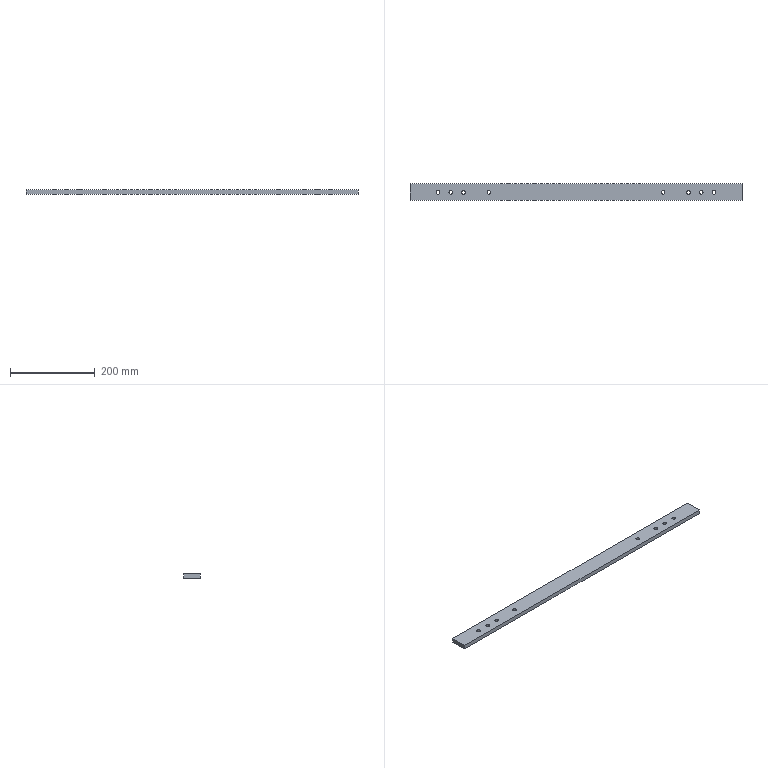Part | SolidWorks | features Extrusion 1, HoleWzd 1 | 1 solid | 22 faces | box 782 x 40 x 10 mm | volume 308260 mm3 | cylinder 16 | plane 6 | commonest cylinder face diameters 8.5 x16
STEP:
#1=CARTESIAN_POINT('',(-320.75,-0.78,0.));
#2=VERTEX_POINT('',#1);
#3=CARTESIAN_POINT('',(-329.25,-0.78,0.));
#4=VERTEX_POINT('',#3);
#5=CARTESIAN_POINT('',(-325.,-0.78,0.));
#6=DIRECTION('',(0.,0.,-1.));
#7=DIRECTION('',(-1.,0.,0.));
#8=AXIS2_PLACEMENT_3D('',#5,#6,#7);
#9=CIRCLE('',#8,4.25);
#10=EDGE_CURVE('',#2,#4,#9,.T.);
#11=ORIENTED_EDGE('',*,*,#10,.T.);
#12=CARTESIAN_POINT('',(-329.25,-0.78,10.));
#13=VERTEX_POINT('',#12);
#14=CARTESIAN_POINT('',(-329.25,-0.78,10.));
#15=DIRECTION('',(0.,0.,1.));
#16=VECTOR('',#15,1000.);
#17=LINE('',#14,#16);
#18=EDGE_CURVE('',#4,#13,#17,.T.);
#19=ORIENTED_EDGE('',*,*,#18,.T.);
#20=CARTESIAN_POINT('',(-320.75,-0.78,10.));
#21=VERTEX_POINT('',#20);
#22=CARTESIAN_POINT('',(-325.,-0.78,10.));
#23=DIRECTION('',(0.,0.,1.));
#24=DIRECTION('',(1.,0.,0.));
#25=AXIS2_PLACEMENT_3D('',#22,#23,#24);
#26=CIRCLE('',#25,4.25);
#27=EDGE_CURVE('',#13,#21,#26,.T.);
#28=ORIENTED_EDGE('',*,*,#27,.T.);
#29=CARTESIAN_POINT('',(-320.75,-0.78,10.));
#30=DIRECTION('',(0.,0.,1.));
#31=VECTOR('',#30,1000.);
#32=LINE('',#29,#31);
#33=EDGE_CURVE('',#2,#21,#32,.T.);
#34=ORIENTED_EDGE('',*,*,#33,.F.);
#35=EDGE_LOOP('',(#11,#19,#28,#34));
#36=FACE_OUTER_BOUND('',#35,.T.);
#37=CARTESIAN_POINT('',(-325.,-0.78,10.));
#38=DIRECTION('',(0.,0.,1.));
#39=DIRECTION('',(1.,0.,0.));
#40=AXIS2_PLACEMENT_3D('',#37,#38,#39);
#41=CYLINDRICAL_SURFACE('',#40,4.25);
#42=ADVANCED_FACE('',(#36),#41,.F.);
#43=CARTESIAN_POINT('',(-290.75,-0.78,0.));
#44=VERTEX_POINT('',#43);
#45=CARTESIAN_POINT('',(-299.25,-0.78,0.));
#46=VERTEX_POINT('',#45);
#47=CARTESIAN_POINT('',(-295.,-0.78,0.));
#48=DIRECTION('',(0.,0.,-1.));
#49=DIRECTION('',(-1.,0.,0.));
#50=AXIS2_PLACEMENT_3D('',#47,#48,#49);
#51=CIRCLE('',#50,4.25);
#52=EDGE_CURVE('',#44,#46,#51,.T.);
#53=ORIENTED_EDGE('',*,*,#52,.T.);
#54=CARTESIAN_POINT('',(-299.25,-0.78,10.));
#55=VERTEX_POINT('',#54);
#56=CARTESIAN_POINT('',(-299.25,-0.78,10.));
#57=DIRECTION('',(0.,0.,1.));
#58=VECTOR('',#57,1000.);
#59=LINE('',#56,#58);
#60=EDGE_CURVE('',#46,#55,#59,.T.);
#61=ORIENTED_EDGE('',*,*,#60,.T.);
#62=CARTESIAN_POINT('',(-290.75,-0.78,10.));
#63=VERTEX_POINT('',#62);
#64=CARTESIAN_POINT('',(-295.,-0.78,10.));
#65=DIRECTION('',(0.,0.,1.));
#66=DIRECTION('',(1.,0.,0.));
#67=AXIS2_PLACEMENT_3D('',#64,#65,#66);
#68=CIRCLE('',#67,4.25);
#69=EDGE_CURVE('',#55,#63,#68,.T.);
#70=ORIENTED_EDGE('',*,*,#69,.T.);
#71=CARTESIAN_POINT('',(-290.75,-0.78,10.));
#72=DIRECTION('',(0.,0.,1.));
#73=VECTOR('',#72,1000.);
#74=LINE('',#71,#73);
#75=EDGE_CURVE('',#44,#63,#74,.T.);
#76=ORIENTED_EDGE('',*,*,#75,.F.);
#77=EDGE_LOOP('',(#53,#61,#70,#76));
#78=FACE_OUTER_BOUND('',#77,.T.);
#79=CARTESIAN_POINT('',(-295.,-0.78,10.));
#80=DIRECTION('',(0.,0.,1.));
#81=DIRECTION('',(1.,0.,0.));
#82=AXIS2_PLACEMENT_3D('',#79,#80,#81);
#83=CYLINDRICAL_SURFACE('',#82,4.25);
#84=ADVANCED_FACE('',(#78),#83,.F.);
#85=CARTESIAN_POINT('',(-260.75,-0.78,0.));
#86=VERTEX_POINT('',#85);
#87=CARTESIAN_POINT('',(-269.25,-0.78,0.));
#88=VERTEX_POINT('',#87);
#89=CARTESIAN_POINT('',(-265.,-0.78,0.));
#90=DIRECTION('',(0.,0.,-1.));
#91=DIRECTION('',(-1.,0.,0.));
#92=AXIS2_PLACEMENT_3D('',#89,#90,#91);
#93=CIRCLE('',#92,4.25);
#94=EDGE_CURVE('',#86,#88,#93,.T.);
#95=ORIENTED_EDGE('',*,*,#94,.T.);
#96=CARTESIAN_POINT('',(-269.25,-0.78,10.));
#97=VERTEX_POINT('',#96);
#98=CARTESIAN_POINT('',(-269.25,-0.78,10.));
#99=DIRECTION('',(0.,0.,1.));
#100=VECTOR('',#99,1000.);
#101=LINE('',#98,#100);
#102=EDGE_CURVE('',#88,#97,#101,.T.);
#103=ORIENTED_EDGE('',*,*,#102,.T.);
#104=CARTESIAN_POINT('',(-260.75,-0.78,10.));
#105=VERTEX_POINT('',#104);
#106=CARTESIAN_POINT('',(-265.,-0.78,10.));
#107=DIRECTION('',(0.,0.,1.));
#108=DIRECTION('',(1.,0.,0.));
#109=AXIS2_PLACEMENT_3D('',#106,#107,#108);
#110=CIRCLE('',#109,4.25);
#111=EDGE_CURVE('',#97,#105,#110,.T.);
#112=ORIENTED_EDGE('',*,*,#111,.T.);
#113=CARTESIAN_POINT('',(-260.75,-0.78,10.));
#114=DIRECTION('',(0.,0.,1.));
#115=VECTOR('',#114,1000.);
#116=LINE('',#113,#115);
#117=EDGE_CURVE('',#86,#105,#116,.T.);
#118=ORIENTED_EDGE('',*,*,#117,.F.);
#119=EDGE_LOOP('',(#95,#103,#112,#118));
#120=FACE_OUTER_BOUND('',#119,.T.);
#121=CARTESIAN_POINT('',(-265.,-0.78,10.));
#122=DIRECTION('',(0.,0.,1.));
#123=DIRECTION('',(1.,0.,0.));
#124=AXIS2_PLACEMENT_3D('',#121,#122,#123);
#125=CYLINDRICAL_SURFACE('',#124,4.25);
#126=ADVANCED_FACE('',(#120),#125,.F.);
#127=CARTESIAN_POINT('',(-200.75,-0.78,0.));
#128=VERTEX_POINT('',#127);
#129=CARTESIAN_POINT('',(-209.25,-0.78,0.));
#130=VERTEX_POINT('',#129);
#131=CARTESIAN_POINT('',(-205.,-0.78,0.));
#132=DIRECTION('',(0.,0.,-1.));
#133=DIRECTION('',(-1.,0.,0.));
#134=AXIS2_PLACEMENT_3D('',#131,#132,#133);
#135=CIRCLE('',#134,4.25);
#136=EDGE_CURVE('',#128,#130,#135,.T.);
#137=ORIENTED_EDGE('',*,*,#136,.T.);
#138=CARTESIAN_POINT('',(-209.25,-0.78,10.));
#139=VERTEX_POINT('',#138);
#140=CARTESIAN_POINT('',(-209.25,-0.78,10.));
#141=DIRECTION('',(0.,0.,1.));
#142=VECTOR('',#141,1000.);
#143=LINE('',#140,#142);
#144=EDGE_CURVE('',#130,#139,#143,.T.);
#145=ORIENTED_EDGE('',*,*,#144,.T.);
#146=CARTESIAN_POINT('',(-200.75,-0.78,10.));
#147=VERTEX_POINT('',#146);
#148=CARTESIAN_POINT('',(-205.,-0.78,10.));
#149=DIRECTION('',(0.,0.,1.));
#150=DIRECTION('',(1.,0.,0.));
#151=AXIS2_PLACEMENT_3D('',#148,#149,#150);
#152=CIRCLE('',#151,4.25);
#153=EDGE_CURVE('',#139,#147,#152,.T.);
#154=ORIENTED_EDGE('',*,*,#153,.T.);
#155=CARTESIAN_POINT('',(-200.75,-0.78,10.));
#156=DIRECTION('',(0.,0.,1.));
#157=VECTOR('',#156,1000.);
#158=LINE('',#155,#157);
#159=EDGE_CURVE('',#128,#147,#158,.T.);
#160=ORIENTED_EDGE('',*,*,#159,.F.);
#161=EDGE_LOOP('',(#137,#145,#154,#160));
#162=FACE_OUTER_BOUND('',#161,.T.);
#163=CARTESIAN_POINT('',(-205.,-0.78,10.));
#164=DIRECTION('',(0.,0.,1.));
#165=DIRECTION('',(1.,0.,0.));
#166=AXIS2_PLACEMENT_3D('',#163,#164,#165);
#167=CYLINDRICAL_SURFACE('',#166,4.25);
#168=ADVANCED_FACE('',(#162),#167,.F.);
#169=CARTESIAN_POINT('',(209.25,-0.78,0.));
#170=VERTEX_POINT('',#169);
#171=CARTESIAN_POINT('',(200.75,-0.78,0.));
#172=VERTEX_POINT('',#171);
#173=CARTESIAN_POINT('',(205.,-0.78,0.));
#174=DIRECTION('',(0.,0.,-1.));
#175=DIRECTION('',(-1.,0.,0.));
#176=AXIS2_PLACEMENT_3D('',#173,#174,#175);
#177=CIRCLE('',#176,4.25);
#178=EDGE_CURVE('',#170,#172,#177,.T.);
#179=ORIENTED_EDGE('',*,*,#178,.T.);
#180=CARTESIAN_POINT('',(200.75,-0.78,10.));
#181=VERTEX_POINT('',#180);
#182=CARTESIAN_POINT('',(200.75,-0.78,10.));
#183=DIRECTION('',(0.,0.,1.));
#184=VECTOR('',#183,1000.);
#185=LINE('',#182,#184);
#186=EDGE_CURVE('',#172,#181,#185,.T.);
#187=ORIENTED_EDGE('',*,*,#186,.T.);
#188=CARTESIAN_POINT('',(209.25,-0.78,10.));
#189=VERTEX_POINT('',#188);
#190=CARTESIAN_POINT('',(205.,-0.78,10.));
#191=DIRECTION('',(0.,0.,1.));
#192=DIRECTION('',(1.,0.,0.));
#193=AXIS2_PLACEMENT_3D('',#190,#191,#192);
#194=CIRCLE('',#193,4.25);
#195=EDGE_CURVE('',#181,#189,#194,.T.);
#196=ORIENTED_EDGE('',*,*,#195,.T.);
#197=CARTESIAN_POINT('',(209.25,-0.78,10.));
#198=DIRECTION('',(0.,0.,1.));
#199=VECTOR('',#198,1000.);
#200=LINE('',#197,#199);
#201=EDGE_CURVE('',#170,#189,#200,.T.);
#202=ORIENTED_EDGE('',*,*,#201,.F.);
#203=EDGE_LOOP('',(#179,#187,#196,#202));
#204=FACE_OUTER_BOUND('',#203,.T.);
#205=CARTESIAN_POINT('',(205.,-0.78,10.));
#206=DIRECTION('',(0.,0.,1.));
#207=DIRECTION('',(1.,0.,0.));
#208=AXIS2_PLACEMENT_3D('',#205,#206,#207);
#209=CYLINDRICAL_SURFACE('',#208,4.25);
#210=ADVANCED_FACE('',(#204),#209,.F.);
#211=CARTESIAN_POINT('',(269.25,-0.78,0.));
#212=VERTEX_POINT('',#211);
#213=CARTESIAN_POINT('',(260.75,-0.78,0.));
#214=VERTEX_POINT('',#213);
#215=CARTESIAN_POINT('',(265.,-0.78,0.));
#216=DIRECTION('',(0.,0.,-1.));
#217=DIRECTION('',(-1.,0.,0.));
#218=AXIS2_PLACEMENT_3D('',#215,#216,#217);
#219=CIRCLE('',#218,4.25);
#220=EDGE_CURVE('',#212,#214,#219,.T.);
#221=ORIENTED_EDGE('',*,*,#220,.T.);
#222=CARTESIAN_POINT('',(260.75,-0.78,10.));
#223=VERTEX_POINT('',#222);
#224=CARTESIAN_POINT('',(260.75,-0.78,10.));
#225=DIRECTION('',(0.,0.,1.));
#226=VECTOR('',#225,1000.);
#227=LINE('',#224,#226);
#228=EDGE_CURVE('',#214,#223,#227,.T.);
#229=ORIENTED_EDGE('',*,*,#228,.T.);
#230=CARTESIAN_POINT('',(269.25,-0.78,10.));
#231=VERTEX_POINT('',#230);
#232=CARTESIAN_POINT('',(265.,-0.78,10.));
#233=DIRECTION('',(0.,0.,1.));
#234=DIRECTION('',(1.,0.,0.));
#235=AXIS2_PLACEMENT_3D('',#232,#233,#234);
#236=CIRCLE('',#235,4.25);
#237=EDGE_CURVE('',#223,#231,#236,.T.);
#238=ORIENTED_EDGE('',*,*,#237,.T.);
#239=CARTESIAN_POINT('',(269.25,-0.78,10.));
#240=DIRECTION('',(0.,0.,1.));
#241=VECTOR('',#240,1000.);
#242=LINE('',#239,#241);
#243=EDGE_CURVE('',#212,#231,#242,.T.);
#244=ORIENTED_EDGE('',*,*,#243,.F.);
#245=EDGE_LOOP('',(#221,#229,#238,#244));
#246=FACE_OUTER_BOUND('',#245,.T.);
#247=CARTESIAN_POINT('',(265.,-0.78,10.));
#248=DIRECTION('',(0.,0.,1.));
#249=DIRECTION('',(1.,0.,0.));
#250=AXIS2_PLACEMENT_3D('',#247,#248,#249);
#251=CYLINDRICAL_SURFACE('',#250,4.25);
#252=ADVANCED_FACE('',(#246),#251,.F.);
#253=CARTESIAN_POINT('',(299.25,-0.78,0.));
#254=VERTEX_POINT('',#253);
#255=CARTESIAN_POINT('',(290.75,-0.78,0.));
#256=VERTEX_POINT('',#255);
#257=CARTESIAN_POINT('',(295.,-0.78,0.));
#258=DIRECTION('',(0.,0.,-1.));
#259=DIRECTION('',(-1.,0.,0.));
#260=AXIS2_PLACEMENT_3D('',#257,#258,#259);
#261=CIRCLE('',#260,4.25);
#262=EDGE_CURVE('',#254,#256,#261,.T.);
#263=ORIENTED_EDGE('',*,*,#262,.T.);
#264=CARTESIAN_POINT('',(290.75,-0.78,10.));
#265=VERTEX_POINT('',#264);
#266=CARTESIAN_POINT('',(290.75,-0.78,10.));
#267=DIRECTION('',(0.,0.,1.));
#268=VECTOR('',#267,1000.);
#269=LINE('',#266,#268);
#270=EDGE_CURVE('',#256,#265,#269,.T.);
#271=ORIENTED_EDGE('',*,*,#270,.T.);
#272=CARTESIAN_POINT('',(299.25,-0.78,10.));
#273=VERTEX_POINT('',#272);
#274=CARTESIAN_POINT('',(295.,-0.78,10.));
#275=DIRECTION('',(0.,0.,1.));
#276=DIRECTION('',(1.,0.,0.));
#277=AXIS2_PLACEMENT_3D('',#274,#275,#276);
#278=CIRCLE('',#277,4.25);
#279=EDGE_CURVE('',#265,#273,#278,.T.);
#280=ORIENTED_EDGE('',*,*,#279,.T.);
#281=CARTESIAN_POINT('',(299.25,-0.78,10.));
#282=DIRECTION('',(0.,0.,1.));
#283=VECTOR('',#282,1000.);
#284=LINE('',#281,#283);
#285=EDGE_CURVE('',#254,#273,#284,.T.);
#286=ORIENTED_EDGE('',*,*,#285,.F.);
#287=EDGE_LOOP('',(#263,#271,#280,#286));
#288=FACE_OUTER_BOUND('',#287,.T.);
#289=CARTESIAN_POINT('',(295.,-0.78,10.));
#290=DIRECTION('',(0.,0.,1.));
#291=DIRECTION('',(1.,0.,0.));
#292=AXIS2_PLACEMENT_3D('',#289,#290,#291);
#293=CYLINDRICAL_SURFACE('',#292,4.25);
#294=ADVANCED_FACE('',(#288),#293,.F.);
#295=CARTESIAN_POINT('',(329.25,-0.78,0.));
#296=VERTEX_POINT('',#295);
#297=CARTESIAN_POINT('',(320.75,-0.78,0.));
#298=VERTEX_POINT('',#297);
#299=CARTESIAN_POINT('',(325.,-0.78,0.));
#300=DIRECTION('',(0.,0.,-1.));
#301=DIRECTION('',(-1.,0.,0.));
#302=AXIS2_PLACEMENT_3D('',#299,#300,#301);
#303=CIRCLE('',#302,4.25);
#304=EDGE_CURVE('',#296,#298,#303,.T.);
#305=ORIENTED_EDGE('',*,*,#304,.T.);
#306=CARTESIAN_POINT('',(320.75,-0.78,10.));
#307=VERTEX_POINT('',#306);
#308=CARTESIAN_POINT('',(320.75,-0.78,10.));
#309=DIRECTION('',(0.,0.,1.));
#310=VECTOR('',#309,1000.);
#311=LINE('',#308,#310);
#312=EDGE_CURVE('',#298,#307,#311,.T.);
#313=ORIENTED_EDGE('',*,*,#312,.T.);
#314=CARTESIAN_POINT('',(329.25,-0.78,10.));
#315=VERTEX_POINT('',#314);
#316=CARTESIAN_POINT('',(325.,-0.78,10.));
#317=DIRECTION('',(0.,0.,1.));
#318=DIRECTION('',(1.,0.,0.));
#319=AXIS2_PLACEMENT_3D('',#316,#317,#318);
#320=CIRCLE('',#319,4.25);
#321=EDGE_CURVE('',#307,#315,#320,.T.);
#322=ORIENTED_EDGE('',*,*,#321,.T.);
#323=CARTESIAN_POINT('',(329.25,-0.78,10.));
#324=DIRECTION('',(0.,0.,1.));
#325=VECTOR('',#324,1000.);
#326=LINE('',#323,#325);
#327=EDGE_CURVE('',#296,#315,#326,.T.);
#328=ORIENTED_EDGE('',*,*,#327,.F.);
#329=EDGE_LOOP('',(#305,#313,#322,#328));
#330=FACE_OUTER_BOUND('',#329,.T.);
#331=CARTESIAN_POINT('',(325.,-0.78,10.));
#332=DIRECTION('',(0.,0.,1.));
#333=DIRECTION('',(1.,0.,0.));
#334=AXIS2_PLACEMENT_3D('',#331,#332,#333);
#335=CYLINDRICAL_SURFACE('',#334,4.25);
#336=ADVANCED_FACE('',(#330),#335,.F.);
#337=CARTESIAN_POINT('',(-391.,20.,0.));
#338=VERTEX_POINT('',#337);
#339=CARTESIAN_POINT('',(-391.,-20.,0.));
#340=VERTEX_POINT('',#339);
#341=CARTESIAN_POINT('',(-391.,20.,0.));
#342=DIRECTION('',(0.,-1.,0.));
#343=VECTOR('',#342,1000.);
#344=LINE('',#341,#343);
#345=EDGE_CURVE('',#338,#340,#344,.T.);
#346=ORIENTED_EDGE('',*,*,#345,.T.);
#347=CARTESIAN_POINT('',(-391.,-20.,10.));
#348=VERTEX_POINT('',#347);
#349=CARTESIAN_POINT('',(-391.,-20.,10.));
#350=DIRECTION('',(0.,0.,-1.));
#351=VECTOR('',#350,1000.);
#352=LINE('',#349,#351);
#353=EDGE_CURVE('',#348,#340,#352,.T.);
#354=ORIENTED_EDGE('',*,*,#353,.F.);
#355=CARTESIAN_POINT('',(-391.,20.,10.));
#356=VERTEX_POINT('',#355);
#357=CARTESIAN_POINT('',(-391.,20.,10.));
#358=DIRECTION('',(0.,-1.,0.));
#359=VECTOR('',#358,1000.);
#360=LINE('',#357,#359);
#361=EDGE_CURVE('',#356,#348,#360,.T.);
#362=ORIENTED_EDGE('',*,*,#361,.F.);
#363=CARTESIAN_POINT('',(-391.,20.,10.));
#364=DIRECTION('',(0.,0.,-1.));
#365=VECTOR('',#364,1000.);
#366=LINE('',#363,#365);
#367=EDGE_CURVE('',#356,#338,#366,.T.);
#368=ORIENTED_EDGE('',*,*,#367,.T.);
#369=EDGE_LOOP('',(#346,#354,#362,#368));
#370=FACE_OUTER_BOUND('',#369,.T.);
#371=CARTESIAN_POINT('',(-391.,20.,10.));
#372=DIRECTION('',(1.,0.,0.));
#373=DIRECTION('',(0.,0.,-1.));
#374=AXIS2_PLACEMENT_3D('',#371,#372,#373);
#375=PLANE('',#374);
#376=ADVANCED_FACE('',(#370),#375,.F.);
#377=CARTESIAN_POINT('',(391.,-20.,0.));
#378=VERTEX_POINT('',#377);
#379=CARTESIAN_POINT('',(391.,-20.,0.));
#380=DIRECTION('',(1.,0.,0.));
#381=VECTOR('',#380,1000.);
#382=LINE('',#379,#381);
#383=EDGE_CURVE('',#340,#378,#382,.T.);
#384=ORIENTED_EDGE('',*,*,#383,.T.);
#385=CARTESIAN_POINT('',(391.,-20.,10.));
#386=VERTEX_POINT('',#385);
#387=CARTESIAN_POINT('',(391.,-20.,10.));
#388=DIRECTION('',(0.,0.,-1.));
#389=VECTOR('',#388,1000.);
#390=LINE('',#387,#389);
#391=EDGE_CURVE('',#386,#378,#390,.T.);
#392=ORIENTED_EDGE('',*,*,#391,.F.);
#393=CARTESIAN_POINT('',(391.,-20.,10.));
#394=DIRECTION('',(1.,0.,0.));
#395=VECTOR('',#394,1000.);
#396=LINE('',#393,#395);
#397=EDGE_CURVE('',#348,#386,#396,.T.);
#398=ORIENTED_EDGE('',*,*,#397,.F.);
#399=ORIENTED_EDGE('',*,*,#353,.T.);
#400=EDGE_LOOP('',(#384,#392,#398,#399));
#401=FACE_OUTER_BOUND('',#400,.T.);
#402=CARTESIAN_POINT('',(391.,-20.,10.));
#403=DIRECTION('',(0.,1.,0.));
#404=DIRECTION('',(-1.,0.,0.));
#405=AXIS2_PLACEMENT_3D('',#402,#403,#404);
#406=PLANE('',#405);
#407=ADVANCED_FACE('',(#401),#406,.F.);
#408=CARTESIAN_POINT('',(391.,20.,0.));
#409=VERTEX_POINT('',#408);
#410=CARTESIAN_POINT('',(391.,20.,0.));
#411=DIRECTION('',(0.,1.,0.));
#412=VECTOR('',#411,1000.);
#413=LINE('',#410,#412);
#414=EDGE_CURVE('',#378,#409,#413,.T.);
#415=ORIENTED_EDGE('',*,*,#414,.T.);
#416=CARTESIAN_POINT('',(391.,20.,10.));
#417=VERTEX_POINT('',#416);
#418=CARTESIAN_POINT('',(391.,20.,10.));
#419=DIRECTION('',(0.,0.,-1.));
#420=VECTOR('',#419,1000.);
#421=LINE('',#418,#420);
#422=EDGE_CURVE('',#417,#409,#421,.T.);
#423=ORIENTED_EDGE('',*,*,#422,.F.);
#424=CARTESIAN_POINT('',(391.,20.,10.));
#425=DIRECTION('',(0.,1.,0.));
#426=VECTOR('',#425,1000.);
#427=LINE('',#424,#426);
#428=EDGE_CURVE('',#386,#417,#427,.T.);
#429=ORIENTED_EDGE('',*,*,#428,.F.);
#430=ORIENTED_EDGE('',*,*,#391,.T.);
#431=EDGE_LOOP('',(#415,#423,#429,#430));
#432=FACE_OUTER_BOUND('',#431,.T.);
#433=CARTESIAN_POINT('',(391.,20.,10.));
#434=DIRECTION('',(-1.,0.,0.));
#435=DIRECTION('',(0.,0.,1.));
#436=AXIS2_PLACEMENT_3D('',#433,#434,#435);
#437=PLANE('',#436);
#438=ADVANCED_FACE('',(#432),#437,.F.);
#439=CARTESIAN_POINT('',(391.,20.,0.));
#440=DIRECTION('',(-1.,0.,0.));
#441=VECTOR('',#440,1000.);
#442=LINE('',#439,#441);
#443=EDGE_CURVE('',#409,#338,#442,.T.);
#444=ORIENTED_EDGE('',*,*,#443,.T.);
#445=ORIENTED_EDGE('',*,*,#367,.F.);
#446=CARTESIAN_POINT('',(391.,20.,10.));
#447=DIRECTION('',(-1.,0.,0.));
#448=VECTOR('',#447,1000.);
#449=LINE('',#446,#448);
#450=EDGE_CURVE('',#417,#356,#449,.T.);
#451=ORIENTED_EDGE('',*,*,#450,.F.);
#452=ORIENTED_EDGE('',*,*,#422,.T.);
#453=EDGE_LOOP('',(#444,#445,#451,#452));
#454=FACE_OUTER_BOUND('',#453,.T.);
#455=CARTESIAN_POINT('',(391.,20.,10.));
#456=DIRECTION('',(0.,-1.,0.));
#457=DIRECTION('',(1.,0.,0.));
#458=AXIS2_PLACEMENT_3D('',#455,#456,#457);
#459=PLANE('',#458);
#460=ADVANCED_FACE('',(#454),#459,.F.);
#461=CARTESIAN_POINT('',(-325.,-0.78,10.));
#462=DIRECTION('',(0.,0.,1.));
#463=DIRECTION('',(1.,0.,0.));
#464=AXIS2_PLACEMENT_3D('',#461,#462,#463);
#465=CIRCLE('',#464,4.25);
#466=EDGE_CURVE('',#21,#13,#465,.T.);
#467=ORIENTED_EDGE('',*,*,#466,.F.);
#468=ORIENTED_EDGE('',*,*,#27,.F.);
#469=EDGE_LOOP('',(#467,#468));
#470=FACE_BOUND('',#469,.T.);
#471=CARTESIAN_POINT('',(-295.,-0.78,10.));
#472=DIRECTION('',(0.,0.,1.));
#473=DIRECTION('',(1.,0.,0.));
#474=AXIS2_PLACEMENT_3D('',#471,#472,#473);
#475=CIRCLE('',#474,4.25);
#476=EDGE_CURVE('',#63,#55,#475,.T.);
#477=ORIENTED_EDGE('',*,*,#476,.F.);
#478=ORIENTED_EDGE('',*,*,#69,.F.);
#479=EDGE_LOOP('',(#477,#478));
#480=FACE_BOUND('',#479,.T.);
#481=CARTESIAN_POINT('',(-265.,-0.78,10.));
#482=DIRECTION('',(0.,0.,1.));
#483=DIRECTION('',(1.,0.,0.));
#484=AXIS2_PLACEMENT_3D('',#481,#482,#483);
#485=CIRCLE('',#484,4.25);
#486=EDGE_CURVE('',#105,#97,#485,.T.);
#487=ORIENTED_EDGE('',*,*,#486,.F.);
#488=ORIENTED_EDGE('',*,*,#111,.F.);
#489=EDGE_LOOP('',(#487,#488));
#490=FACE_BOUND('',#489,.T.);
#491=CARTESIAN_POINT('',(-205.,-0.78,10.));
#492=DIRECTION('',(0.,0.,1.));
#493=DIRECTION('',(1.,0.,0.));
#494=AXIS2_PLACEMENT_3D('',#491,#492,#493);
#495=CIRCLE('',#494,4.25);
#496=EDGE_CURVE('',#147,#139,#495,.T.);
#497=ORIENTED_EDGE('',*,*,#496,.F.);
#498=ORIENTED_EDGE('',*,*,#153,.F.);
#499=EDGE_LOOP('',(#497,#498));
#500=FACE_BOUND('',#499,.T.);
#501=CARTESIAN_POINT('',(205.,-0.78,10.));
#502=DIRECTION('',(0.,0.,1.));
#503=DIRECTION('',(1.,0.,0.));
#504=AXIS2_PLACEMENT_3D('',#501,#502,#503);
#505=CIRCLE('',#504,4.25);
#506=EDGE_CURVE('',#189,#181,#505,.T.);
#507=ORIENTED_EDGE('',*,*,#506,.F.);
#508=ORIENTED_EDGE('',*,*,#195,.F.);
#509=EDGE_LOOP('',(#507,#508));
#510=FACE_BOUND('',#509,.T.);
#511=CARTESIAN_POINT('',(265.,-0.78,10.));
#512=DIRECTION('',(0.,0.,1.));
#513=DIRECTION('',(1.,0.,0.));
#514=AXIS2_PLACEMENT_3D('',#511,#512,#513);
#515=CIRCLE('',#514,4.25);
#516=EDGE_CURVE('',#231,#223,#515,.T.);
#517=ORIENTED_EDGE('',*,*,#516,.F.);
#518=ORIENTED_EDGE('',*,*,#237,.F.);
#519=EDGE_LOOP('',(#517,#518));
#520=FACE_BOUND('',#519,.T.);
#521=CARTESIAN_POINT('',(295.,-0.78,10.));
#522=DIRECTION('',(0.,0.,1.));
#523=DIRECTION('',(1.,0.,0.));
#524=AXIS2_PLACEMENT_3D('',#521,#522,#523);
#525=CIRCLE('',#524,4.25);
#526=EDGE_CURVE('',#273,#265,#525,.T.);
#527=ORIENTED_EDGE('',*,*,#526,.F.);
#528=ORIENTED_EDGE('',*,*,#279,.F.);
#529=EDGE_LOOP('',(#527,#528));
#530=FACE_BOUND('',#529,.T.);
#531=CARTESIAN_POINT('',(325.,-0.78,10.));
#532=DIRECTION('',(0.,0.,1.));
#533=DIRECTION('',(1.,0.,0.));
#534=AXIS2_PLACEMENT_3D('',#531,#532,#533);
#535=CIRCLE('',#534,4.25);
#536=EDGE_CURVE('',#315,#307,#535,.T.);
#537=ORIENTED_EDGE('',*,*,#536,.F.);
#538=ORIENTED_EDGE('',*,*,#321,.F.);
#539=EDGE_LOOP('',(#537,#538));
#540=FACE_BOUND('',#539,.T.);
#541=ORIENTED_EDGE('',*,*,#361,.T.);
#542=ORIENTED_EDGE('',*,*,#397,.T.);
#543=ORIENTED_EDGE('',*,*,#428,.T.);
#544=ORIENTED_EDGE('',*,*,#450,.T.);
#545=EDGE_LOOP('',(#541,#542,#543,#544));
#546=FACE_OUTER_BOUND('',#545,.T.);
#547=CARTESIAN_POINT('',(0.,0.,10.));
#548=DIRECTION('',(0.,0.,-1.));
#549=DIRECTION('',(-1.,0.,0.));
#550=AXIS2_PLACEMENT_3D('',#547,#548,#549);
#551=PLANE('',#550);
#552=ADVANCED_FACE('',(#470,#480,#490,#500,#510,#520,#530,#540,#546),#551,.F.);
#553=ORIENTED_EDGE('',*,*,#10,.F.);
#554=CARTESIAN_POINT('',(-325.,-0.78,0.));
#555=DIRECTION('',(0.,0.,-1.));
#556=DIRECTION('',(-1.,0.,0.));
#557=AXIS2_PLACEMENT_3D('',#554,#555,#556);
#558=CIRCLE('',#557,4.25);
#559=EDGE_CURVE('',#4,#2,#558,.T.);
#560=ORIENTED_EDGE('',*,*,#559,.F.);
#561=EDGE_LOOP('',(#553,#560));
#562=FACE_BOUND('',#561,.T.);
#563=ORIENTED_EDGE('',*,*,#52,.F.);
#564=CARTESIAN_POINT('',(-295.,-0.78,0.));
#565=DIRECTION('',(0.,0.,-1.));
#566=DIRECTION('',(-1.,0.,0.));
#567=AXIS2_PLACEMENT_3D('',#564,#565,#566);
#568=CIRCLE('',#567,4.25);
#569=EDGE_CURVE('',#46,#44,#568,.T.);
#570=ORIENTED_EDGE('',*,*,#569,.F.);
#571=EDGE_LOOP('',(#563,#570));
#572=FACE_BOUND('',#571,.T.);
#573=ORIENTED_EDGE('',*,*,#94,.F.);
#574=CARTESIAN_POINT('',(-265.,-0.78,0.));
#575=DIRECTION('',(0.,0.,-1.));
#576=DIRECTION('',(-1.,0.,0.));
#577=AXIS2_PLACEMENT_3D('',#574,#575,#576);
#578=CIRCLE('',#577,4.25);
#579=EDGE_CURVE('',#88,#86,#578,.T.);
#580=ORIENTED_EDGE('',*,*,#579,.F.);
#581=EDGE_LOOP('',(#573,#580));
#582=FACE_BOUND('',#581,.T.);
#583=ORIENTED_EDGE('',*,*,#136,.F.);
#584=CARTESIAN_POINT('',(-205.,-0.78,0.));
#585=DIRECTION('',(0.,0.,-1.));
#586=DIRECTION('',(-1.,0.,0.));
#587=AXIS2_PLACEMENT_3D('',#584,#585,#586);
#588=CIRCLE('',#587,4.25);
#589=EDGE_CURVE('',#130,#128,#588,.T.);
#590=ORIENTED_EDGE('',*,*,#589,.F.);
#591=EDGE_LOOP('',(#583,#590));
#592=FACE_BOUND('',#591,.T.);
#593=ORIENTED_EDGE('',*,*,#178,.F.);
#594=CARTESIAN_POINT('',(205.,-0.78,0.));
#595=DIRECTION('',(0.,0.,-1.));
#596=DIRECTION('',(-1.,0.,0.));
#597=AXIS2_PLACEMENT_3D('',#594,#595,#596);
#598=CIRCLE('',#597,4.25);
#599=EDGE_CURVE('',#172,#170,#598,.T.);
#600=ORIENTED_EDGE('',*,*,#599,.F.);
#601=EDGE_LOOP('',(#593,#600));
#602=FACE_BOUND('',#601,.T.);
#603=ORIENTED_EDGE('',*,*,#220,.F.);
#604=CARTESIAN_POINT('',(265.,-0.78,0.));
#605=DIRECTION('',(0.,0.,-1.));
#606=DIRECTION('',(-1.,0.,0.));
#607=AXIS2_PLACEMENT_3D('',#604,#605,#606);
#608=CIRCLE('',#607,4.25);
#609=EDGE_CURVE('',#214,#212,#608,.T.);
#610=ORIENTED_EDGE('',*,*,#609,.F.);
#611=EDGE_LOOP('',(#603,#610));
#612=FACE_BOUND('',#611,.T.);
#613=ORIENTED_EDGE('',*,*,#262,.F.);
#614=CARTESIAN_POINT('',(295.,-0.78,0.));
#615=DIRECTION('',(0.,0.,-1.));
#616=DIRECTION('',(-1.,0.,0.));
#617=AXIS2_PLACEMENT_3D('',#614,#615,#616);
#618=CIRCLE('',#617,4.25);
#619=EDGE_CURVE('',#256,#254,#618,.T.);
#620=ORIENTED_EDGE('',*,*,#619,.F.);
#621=EDGE_LOOP('',(#613,#620));
#622=FACE_BOUND('',#621,.T.);
#623=ORIENTED_EDGE('',*,*,#304,.F.);
#624=CARTESIAN_POINT('',(325.,-0.78,0.));
#625=DIRECTION('',(0.,0.,-1.));
#626=DIRECTION('',(-1.,0.,0.));
#627=AXIS2_PLACEMENT_3D('',#624,#625,#626);
#628=CIRCLE('',#627,4.25);
#629=EDGE_CURVE('',#298,#296,#628,.T.);
#630=ORIENTED_EDGE('',*,*,#629,.F.);
#631=EDGE_LOOP('',(#623,#630));
#632=FACE_BOUND('',#631,.T.);
#633=ORIENTED_EDGE('',*,*,#345,.F.);
#634=ORIENTED_EDGE('',*,*,#443,.F.);
#635=ORIENTED_EDGE('',*,*,#414,.F.);
#636=ORIENTED_EDGE('',*,*,#383,.F.);
#637=EDGE_LOOP('',(#633,#634,#635,#636));
#638=FACE_OUTER_BOUND('',#637,.T.);
#639=CARTESIAN_POINT('',(0.,0.,0.));
#640=DIRECTION('',(0.,0.,-1.));
#641=DIRECTION('',(-1.,0.,0.));
#642=AXIS2_PLACEMENT_3D('',#639,#640,#641);
#643=PLANE('',#642);
#644=ADVANCED_FACE('',(#562,#572,#582,#592,#602,#612,#622,#632,#638),#643,.T.);
#645=ORIENTED_EDGE('',*,*,#312,.F.);
#646=ORIENTED_EDGE('',*,*,#629,.T.);
#647=ORIENTED_EDGE('',*,*,#327,.T.);
#648=ORIENTED_EDGE('',*,*,#536,.T.);
#649=EDGE_LOOP('',(#645,#646,#647,#648));
#650=FACE_OUTER_BOUND('',#649,.T.);
#651=CARTESIAN_POINT('',(325.,-0.78,10.));
#652=DIRECTION('',(0.,0.,1.));
#653=DIRECTION('',(1.,0.,0.));
#654=AXIS2_PLACEMENT_3D('',#651,#652,#653);
#655=CYLINDRICAL_SURFACE('',#654,4.25);
#656=ADVANCED_FACE('',(#650),#655,.F.);
#657=ORIENTED_EDGE('',*,*,#270,.F.);
#658=ORIENTED_EDGE('',*,*,#619,.T.);
#659=ORIENTED_EDGE('',*,*,#285,.T.);
#660=ORIENTED_EDGE('',*,*,#526,.T.);
#661=EDGE_LOOP('',(#657,#658,#659,#660));
#662=FACE_OUTER_BOUND('',#661,.T.);
#663=CARTESIAN_POINT('',(295.,-0.78,10.));
#664=DIRECTION('',(0.,0.,1.));
#665=DIRECTION('',(1.,0.,0.));
#666=AXIS2_PLACEMENT_3D('',#663,#664,#665);
#667=CYLINDRICAL_SURFACE('',#666,4.25);
#668=ADVANCED_FACE('',(#662),#667,.F.);
#669=ORIENTED_EDGE('',*,*,#228,.F.);
#670=ORIENTED_EDGE('',*,*,#609,.T.);
#671=ORIENTED_EDGE('',*,*,#243,.T.);
#672=ORIENTED_EDGE('',*,*,#516,.T.);
#673=EDGE_LOOP('',(#669,#670,#671,#672));
#674=FACE_OUTER_BOUND('',#673,.T.);
#675=CARTESIAN_POINT('',(265.,-0.78,10.));
#676=DIRECTION('',(0.,0.,1.));
#677=DIRECTION('',(1.,0.,0.));
#678=AXIS2_PLACEMENT_3D('',#675,#676,#677);
#679=CYLINDRICAL_SURFACE('',#678,4.25);
#680=ADVANCED_FACE('',(#674),#679,.F.);
#681=ORIENTED_EDGE('',*,*,#186,.F.);
#682=ORIENTED_EDGE('',*,*,#599,.T.);
#683=ORIENTED_EDGE('',*,*,#201,.T.);
#684=ORIENTED_EDGE('',*,*,#506,.T.);
#685=EDGE_LOOP('',(#681,#682,#683,#684));
#686=FACE_OUTER_BOUND('',#685,.T.);
#687=CARTESIAN_POINT('',(205.,-0.78,10.));
#688=DIRECTION('',(0.,0.,1.));
#689=DIRECTION('',(1.,0.,0.));
#690=AXIS2_PLACEMENT_3D('',#687,#688,#689);
#691=CYLINDRICAL_SURFACE('',#690,4.25);
#692=ADVANCED_FACE('',(#686),#691,.F.);
#693=ORIENTED_EDGE('',*,*,#144,.F.);
#694=ORIENTED_EDGE('',*,*,#589,.T.);
#695=ORIENTED_EDGE('',*,*,#159,.T.);
#696=ORIENTED_EDGE('',*,*,#496,.T.);
#697=EDGE_LOOP('',(#693,#694,#695,#696));
#698=FACE_OUTER_BOUND('',#697,.T.);
#699=CARTESIAN_POINT('',(-205.,-0.78,10.));
#700=DIRECTION('',(0.,0.,1.));
#701=DIRECTION('',(1.,0.,0.));
#702=AXIS2_PLACEMENT_3D('',#699,#700,#701);
#703=CYLINDRICAL_SURFACE('',#702,4.25);
#704=ADVANCED_FACE('',(#698),#703,.F.);
#705=ORIENTED_EDGE('',*,*,#102,.F.);
#706=ORIENTED_EDGE('',*,*,#579,.T.);
#707=ORIENTED_EDGE('',*,*,#117,.T.);
#708=ORIENTED_EDGE('',*,*,#486,.T.);
#709=EDGE_LOOP('',(#705,#706,#707,#708));
#710=FACE_OUTER_BOUND('',#709,.T.);
#711=CARTESIAN_POINT('',(-265.,-0.78,10.));
#712=DIRECTION('',(0.,0.,1.));
#713=DIRECTION('',(1.,0.,0.));
#714=AXIS2_PLACEMENT_3D('',#711,#712,#713);
#715=CYLINDRICAL_SURFACE('',#714,4.25);
#716=ADVANCED_FACE('',(#710),#715,.F.);
#717=ORIENTED_EDGE('',*,*,#60,.F.);
#718=ORIENTED_EDGE('',*,*,#569,.T.);
#719=ORIENTED_EDGE('',*,*,#75,.T.);
#720=ORIENTED_EDGE('',*,*,#476,.T.);
#721=EDGE_LOOP('',(#717,#718,#719,#720));
#722=FACE_OUTER_BOUND('',#721,.T.);
#723=CARTESIAN_POINT('',(-295.,-0.78,10.));
#724=DIRECTION('',(0.,0.,1.));
#725=DIRECTION('',(1.,0.,0.));
#726=AXIS2_PLACEMENT_3D('',#723,#724,#725);
#727=CYLINDRICAL_SURFACE('',#726,4.25);
#728=ADVANCED_FACE('',(#722),#727,.F.);
#729=ORIENTED_EDGE('',*,*,#18,.F.);
#730=ORIENTED_EDGE('',*,*,#559,.T.);
#731=ORIENTED_EDGE('',*,*,#33,.T.);
#732=ORIENTED_EDGE('',*,*,#466,.T.);
#733=EDGE_LOOP('',(#729,#730,#731,#732));
#734=FACE_OUTER_BOUND('',#733,.T.);
#735=CARTESIAN_POINT('',(-325.,-0.78,10.));
#736=DIRECTION('',(0.,0.,1.));
#737=DIRECTION('',(1.,0.,0.));
#738=AXIS2_PLACEMENT_3D('',#735,#736,#737);
#739=CYLINDRICAL_SURFACE('',#738,4.25);
#740=ADVANCED_FACE('',(#734),#739,.F.);
#741=CLOSED_SHELL('',(#42,#84,#126,#168,#210,#252,#294,#336,#376,#407,#438,#460,#552,#644,#656,#668,#680,#692,#704,#716,#728,#740));
#742=MANIFOLD_SOLID_BREP('',#741);
#743=CARTESIAN_POINT('',(0.,0.,0.));
#744=DIRECTION('',(0.,0.,1.));
#745=DIRECTION('',(1.,0.,0.));
#746=AXIS2_PLACEMENT_3D('',#743,#744,#745);
#747=(LENGTH_UNIT()NAMED_UNIT(*)SI_UNIT(.MILLI.,.METRE.));
#748=UNCERTAINTY_MEASURE_WITH_UNIT(LENGTH_MEASURE(0.00001),#747,'','');
#749=(NAMED_UNIT(*)PLANE_ANGLE_UNIT()SI_UNIT($,.RADIAN.));
#750=(NAMED_UNIT(*)SI_UNIT($,.STERADIAN.)SOLID_ANGLE_UNIT());
#751=(GEOMETRIC_REPRESENTATION_CONTEXT(3)GLOBAL_UNCERTAINTY_ASSIGNED_CONTEXT((#748))GLOBAL_UNIT_ASSIGNED_CONTEXT((#747,#749,#750))REPRESENTATION_CONTEXT('',''));
#752=ADVANCED_BREP_SHAPE_REPRESENTATION('',(#742,#746),#751);